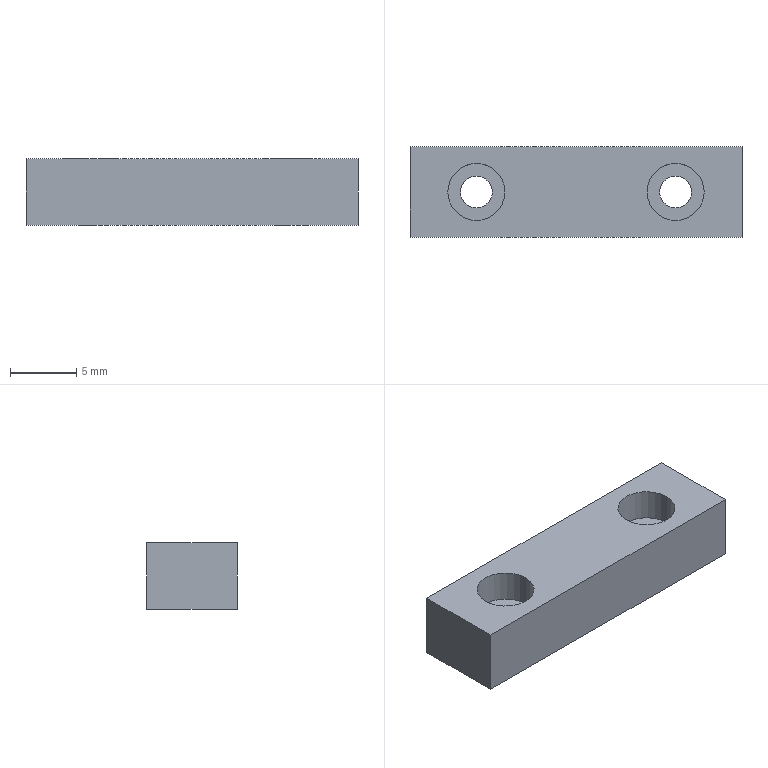Part | SolidWorks | features ICE 2, Extrusion 1 | 1 solid | 16 faces | box 25 x 6.8 x 5 mm | volume 756.77 mm3 | cylinder 8 | plane 8 | commonest cylinder face diameters 2.4 x4 4.3 x4
STEP:
#1=CARTESIAN_POINT('',(9.505,-0.3606,2.6));
#2=VERTEX_POINT('',#1);
#3=CARTESIAN_POINT('',(13.805,-0.3606,2.6));
#4=VERTEX_POINT('',#3);
#5=CARTESIAN_POINT('',(11.655,-0.3606,2.6));
#6=DIRECTION('',(0.,0.,1.));
#7=DIRECTION('',(1.,0.,0.));
#8=AXIS2_PLACEMENT_3D('',#5,#6,#7);
#9=CIRCLE('',#8,2.15);
#10=EDGE_CURVE('',#2,#4,#9,.T.);
#11=ORIENTED_EDGE('',*,*,#10,.F.);
#12=CARTESIAN_POINT('',(9.505,-0.3606,5.));
#13=VERTEX_POINT('',#12);
#14=CARTESIAN_POINT('',(9.505,-0.3606,2.6));
#15=DIRECTION('',(0.,0.,1.));
#16=VECTOR('',#15,1000.);
#17=LINE('',#14,#16);
#18=EDGE_CURVE('',#2,#13,#17,.T.);
#19=ORIENTED_EDGE('',*,*,#18,.T.);
#20=CARTESIAN_POINT('',(13.805,-0.3606,5.));
#21=VERTEX_POINT('',#20);
#22=CARTESIAN_POINT('',(11.655,-0.3606,5.));
#23=DIRECTION('',(0.,0.,1.));
#24=DIRECTION('',(1.,0.,0.));
#25=AXIS2_PLACEMENT_3D('',#22,#23,#24);
#26=CIRCLE('',#25,2.15);
#27=EDGE_CURVE('',#13,#21,#26,.T.);
#28=ORIENTED_EDGE('',*,*,#27,.T.);
#29=CARTESIAN_POINT('',(13.805,-0.3606,2.6));
#30=DIRECTION('',(0.,0.,1.));
#31=VECTOR('',#30,1000.);
#32=LINE('',#29,#31);
#33=EDGE_CURVE('',#4,#21,#32,.T.);
#34=ORIENTED_EDGE('',*,*,#33,.F.);
#35=EDGE_LOOP('',(#11,#19,#28,#34));
#36=FACE_OUTER_BOUND('',#35,.T.);
#37=CARTESIAN_POINT('',(11.655,-0.3606,2.6));
#38=DIRECTION('',(0.,0.,1.));
#39=DIRECTION('',(1.,0.,0.));
#40=AXIS2_PLACEMENT_3D('',#37,#38,#39);
#41=CYLINDRICAL_SURFACE('',#40,2.15);
#42=ADVANCED_FACE('',(#36),#41,.F.);
#43=CARTESIAN_POINT('',(-5.495,-0.3606,2.6));
#44=VERTEX_POINT('',#43);
#45=CARTESIAN_POINT('',(-1.195,-0.3606,2.6));
#46=VERTEX_POINT('',#45);
#47=CARTESIAN_POINT('',(-3.345,-0.3606,2.6));
#48=DIRECTION('',(0.,0.,1.));
#49=DIRECTION('',(1.,0.,0.));
#50=AXIS2_PLACEMENT_3D('',#47,#48,#49);
#51=CIRCLE('',#50,2.15);
#52=EDGE_CURVE('',#44,#46,#51,.T.);
#53=ORIENTED_EDGE('',*,*,#52,.F.);
#54=CARTESIAN_POINT('',(-5.495,-0.3606,5.));
#55=VERTEX_POINT('',#54);
#56=CARTESIAN_POINT('',(-5.495,-0.3606,2.6));
#57=DIRECTION('',(0.,0.,1.));
#58=VECTOR('',#57,1000.);
#59=LINE('',#56,#58);
#60=EDGE_CURVE('',#44,#55,#59,.T.);
#61=ORIENTED_EDGE('',*,*,#60,.T.);
#62=CARTESIAN_POINT('',(-1.195,-0.3606,5.));
#63=VERTEX_POINT('',#62);
#64=CARTESIAN_POINT('',(-3.345,-0.3606,5.));
#65=DIRECTION('',(0.,0.,1.));
#66=DIRECTION('',(1.,0.,0.));
#67=AXIS2_PLACEMENT_3D('',#64,#65,#66);
#68=CIRCLE('',#67,2.15);
#69=EDGE_CURVE('',#55,#63,#68,.T.);
#70=ORIENTED_EDGE('',*,*,#69,.T.);
#71=CARTESIAN_POINT('',(-1.195,-0.3606,2.6));
#72=DIRECTION('',(0.,0.,1.));
#73=VECTOR('',#72,1000.);
#74=LINE('',#71,#73);
#75=EDGE_CURVE('',#46,#63,#74,.T.);
#76=ORIENTED_EDGE('',*,*,#75,.F.);
#77=EDGE_LOOP('',(#53,#61,#70,#76));
#78=FACE_OUTER_BOUND('',#77,.T.);
#79=CARTESIAN_POINT('',(-3.345,-0.3606,2.6));
#80=DIRECTION('',(0.,0.,1.));
#81=DIRECTION('',(1.,0.,0.));
#82=AXIS2_PLACEMENT_3D('',#79,#80,#81);
#83=CYLINDRICAL_SURFACE('',#82,2.15);
#84=ADVANCED_FACE('',(#78),#83,.F.);
#85=CARTESIAN_POINT('',(-2.145,-0.3606,0.));
#86=VERTEX_POINT('',#85);
#87=CARTESIAN_POINT('',(-4.545,-0.3606,0.));
#88=VERTEX_POINT('',#87);
#89=CARTESIAN_POINT('',(-3.345,-0.3606,0.));
#90=DIRECTION('',(0.,0.,-1.));
#91=DIRECTION('',(1.,0.,0.));
#92=AXIS2_PLACEMENT_3D('',#89,#90,#91);
#93=CIRCLE('',#92,1.2);
#94=EDGE_CURVE('',#86,#88,#93,.T.);
#95=ORIENTED_EDGE('',*,*,#94,.T.);
#96=CARTESIAN_POINT('',(-4.545,-0.3606,2.6));
#97=VERTEX_POINT('',#96);
#98=CARTESIAN_POINT('',(-4.545,-0.3606,-0.001));
#99=DIRECTION('',(0.,0.,1.));
#100=VECTOR('',#99,1000.);
#101=LINE('',#98,#100);
#102=EDGE_CURVE('',#88,#97,#101,.T.);
#103=ORIENTED_EDGE('',*,*,#102,.T.);
#104=CARTESIAN_POINT('',(-2.145,-0.3606,2.6));
#105=VERTEX_POINT('',#104);
#106=CARTESIAN_POINT('',(-3.345,-0.3606,2.6));
#107=DIRECTION('',(0.,0.,-1.));
#108=DIRECTION('',(1.,0.,0.));
#109=AXIS2_PLACEMENT_3D('',#106,#107,#108);
#110=CIRCLE('',#109,1.2);
#111=EDGE_CURVE('',#105,#97,#110,.T.);
#112=ORIENTED_EDGE('',*,*,#111,.F.);
#113=CARTESIAN_POINT('',(-2.145,-0.3606,-0.001));
#114=DIRECTION('',(0.,0.,1.));
#115=VECTOR('',#114,1000.);
#116=LINE('',#113,#115);
#117=EDGE_CURVE('',#86,#105,#116,.T.);
#118=ORIENTED_EDGE('',*,*,#117,.F.);
#119=EDGE_LOOP('',(#95,#103,#112,#118));
#120=FACE_OUTER_BOUND('',#119,.T.);
#121=CARTESIAN_POINT('',(-3.345,-0.3606,-0.001));
#122=DIRECTION('',(0.,0.,1.));
#123=DIRECTION('',(1.,0.,0.));
#124=AXIS2_PLACEMENT_3D('',#121,#122,#123);
#125=CYLINDRICAL_SURFACE('',#124,1.2);
#126=ADVANCED_FACE('',(#120),#125,.F.);
#127=CARTESIAN_POINT('',(12.855,-0.3606,0.));
#128=VERTEX_POINT('',#127);
#129=CARTESIAN_POINT('',(10.455,-0.3606,0.));
#130=VERTEX_POINT('',#129);
#131=CARTESIAN_POINT('',(11.655,-0.3606,0.));
#132=DIRECTION('',(0.,0.,-1.));
#133=DIRECTION('',(1.,0.,0.));
#134=AXIS2_PLACEMENT_3D('',#131,#132,#133);
#135=CIRCLE('',#134,1.2);
#136=EDGE_CURVE('',#128,#130,#135,.T.);
#137=ORIENTED_EDGE('',*,*,#136,.T.);
#138=CARTESIAN_POINT('',(10.455,-0.3606,2.6));
#139=VERTEX_POINT('',#138);
#140=CARTESIAN_POINT('',(10.455,-0.3606,-0.001));
#141=DIRECTION('',(0.,0.,1.));
#142=VECTOR('',#141,1000.);
#143=LINE('',#140,#142);
#144=EDGE_CURVE('',#130,#139,#143,.T.);
#145=ORIENTED_EDGE('',*,*,#144,.T.);
#146=CARTESIAN_POINT('',(12.855,-0.3606,2.6));
#147=VERTEX_POINT('',#146);
#148=CARTESIAN_POINT('',(11.655,-0.3606,2.6));
#149=DIRECTION('',(0.,0.,-1.));
#150=DIRECTION('',(1.,0.,0.));
#151=AXIS2_PLACEMENT_3D('',#148,#149,#150);
#152=CIRCLE('',#151,1.2);
#153=EDGE_CURVE('',#147,#139,#152,.T.);
#154=ORIENTED_EDGE('',*,*,#153,.F.);
#155=CARTESIAN_POINT('',(12.855,-0.3606,-0.001));
#156=DIRECTION('',(0.,0.,1.));
#157=VECTOR('',#156,1000.);
#158=LINE('',#155,#157);
#159=EDGE_CURVE('',#128,#147,#158,.T.);
#160=ORIENTED_EDGE('',*,*,#159,.F.);
#161=EDGE_LOOP('',(#137,#145,#154,#160));
#162=FACE_OUTER_BOUND('',#161,.T.);
#163=CARTESIAN_POINT('',(11.655,-0.3606,-0.001));
#164=DIRECTION('',(0.,0.,1.));
#165=DIRECTION('',(1.,0.,0.));
#166=AXIS2_PLACEMENT_3D('',#163,#164,#165);
#167=CYLINDRICAL_SURFACE('',#166,1.2);
#168=ADVANCED_FACE('',(#162),#167,.F.);
#169=ORIENTED_EDGE('',*,*,#144,.F.);
#170=CARTESIAN_POINT('',(11.655,-0.3606,0.));
#171=DIRECTION('',(0.,0.,-1.));
#172=DIRECTION('',(1.,0.,0.));
#173=AXIS2_PLACEMENT_3D('',#170,#171,#172);
#174=CIRCLE('',#173,1.2);
#175=EDGE_CURVE('',#130,#128,#174,.T.);
#176=ORIENTED_EDGE('',*,*,#175,.T.);
#177=ORIENTED_EDGE('',*,*,#159,.T.);
#178=CARTESIAN_POINT('',(11.655,-0.3606,2.6));
#179=DIRECTION('',(0.,0.,-1.));
#180=DIRECTION('',(1.,0.,0.));
#181=AXIS2_PLACEMENT_3D('',#178,#179,#180);
#182=CIRCLE('',#181,1.2);
#183=EDGE_CURVE('',#139,#147,#182,.T.);
#184=ORIENTED_EDGE('',*,*,#183,.F.);
#185=EDGE_LOOP('',(#169,#176,#177,#184));
#186=FACE_OUTER_BOUND('',#185,.T.);
#187=CARTESIAN_POINT('',(11.655,-0.3606,-0.001));
#188=DIRECTION('',(0.,0.,1.));
#189=DIRECTION('',(1.,0.,0.));
#190=AXIS2_PLACEMENT_3D('',#187,#188,#189);
#191=CYLINDRICAL_SURFACE('',#190,1.2);
#192=ADVANCED_FACE('',(#186),#191,.F.);
#193=ORIENTED_EDGE('',*,*,#102,.F.);
#194=CARTESIAN_POINT('',(-3.345,-0.3606,0.));
#195=DIRECTION('',(0.,0.,-1.));
#196=DIRECTION('',(1.,0.,0.));
#197=AXIS2_PLACEMENT_3D('',#194,#195,#196);
#198=CIRCLE('',#197,1.2);
#199=EDGE_CURVE('',#88,#86,#198,.T.);
#200=ORIENTED_EDGE('',*,*,#199,.T.);
#201=ORIENTED_EDGE('',*,*,#117,.T.);
#202=CARTESIAN_POINT('',(-3.345,-0.3606,2.6));
#203=DIRECTION('',(0.,0.,-1.));
#204=DIRECTION('',(1.,0.,0.));
#205=AXIS2_PLACEMENT_3D('',#202,#203,#204);
#206=CIRCLE('',#205,1.2);
#207=EDGE_CURVE('',#97,#105,#206,.T.);
#208=ORIENTED_EDGE('',*,*,#207,.F.);
#209=EDGE_LOOP('',(#193,#200,#201,#208));
#210=FACE_OUTER_BOUND('',#209,.T.);
#211=CARTESIAN_POINT('',(-3.345,-0.3606,-0.001));
#212=DIRECTION('',(0.,0.,1.));
#213=DIRECTION('',(1.,0.,0.));
#214=AXIS2_PLACEMENT_3D('',#211,#212,#213);
#215=CYLINDRICAL_SURFACE('',#214,1.2);
#216=ADVANCED_FACE('',(#210),#215,.F.);
#217=CARTESIAN_POINT('',(-8.345,3.039,0.));
#218=VERTEX_POINT('',#217);
#219=CARTESIAN_POINT('',(-8.345,-3.761,0.));
#220=VERTEX_POINT('',#219);
#221=CARTESIAN_POINT('',(-8.345,3.039,0.));
#222=DIRECTION('',(0.,-1.,0.));
#223=VECTOR('',#222,1000.);
#224=LINE('',#221,#223);
#225=EDGE_CURVE('',#218,#220,#224,.T.);
#226=ORIENTED_EDGE('',*,*,#225,.T.);
#227=CARTESIAN_POINT('',(-8.345,-3.761,5.));
#228=VERTEX_POINT('',#227);
#229=CARTESIAN_POINT('',(-8.345,-3.761,5.));
#230=DIRECTION('',(0.,0.,-1.));
#231=VECTOR('',#230,1000.);
#232=LINE('',#229,#231);
#233=EDGE_CURVE('',#228,#220,#232,.T.);
#234=ORIENTED_EDGE('',*,*,#233,.F.);
#235=CARTESIAN_POINT('',(-8.345,3.039,5.));
#236=VERTEX_POINT('',#235);
#237=CARTESIAN_POINT('',(-8.345,3.039,5.));
#238=DIRECTION('',(0.,-1.,0.));
#239=VECTOR('',#238,1000.);
#240=LINE('',#237,#239);
#241=EDGE_CURVE('',#236,#228,#240,.T.);
#242=ORIENTED_EDGE('',*,*,#241,.F.);
#243=CARTESIAN_POINT('',(-8.345,3.039,5.));
#244=DIRECTION('',(0.,0.,-1.));
#245=VECTOR('',#244,1000.);
#246=LINE('',#243,#245);
#247=EDGE_CURVE('',#236,#218,#246,.T.);
#248=ORIENTED_EDGE('',*,*,#247,.T.);
#249=EDGE_LOOP('',(#226,#234,#242,#248));
#250=FACE_OUTER_BOUND('',#249,.T.);
#251=CARTESIAN_POINT('',(-8.345,3.039,5.));
#252=DIRECTION('',(1.,0.,0.));
#253=DIRECTION('',(0.,0.,-1.));
#254=AXIS2_PLACEMENT_3D('',#251,#252,#253);
#255=PLANE('',#254);
#256=ADVANCED_FACE('',(#250),#255,.F.);
#257=CARTESIAN_POINT('',(16.655,-3.761,0.));
#258=VERTEX_POINT('',#257);
#259=CARTESIAN_POINT('',(-8.345,-3.761,0.));
#260=DIRECTION('',(1.,0.,0.));
#261=VECTOR('',#260,1000.);
#262=LINE('',#259,#261);
#263=EDGE_CURVE('',#220,#258,#262,.T.);
#264=ORIENTED_EDGE('',*,*,#263,.T.);
#265=CARTESIAN_POINT('',(16.655,-3.761,5.));
#266=VERTEX_POINT('',#265);
#267=CARTESIAN_POINT('',(16.655,-3.761,5.));
#268=DIRECTION('',(0.,0.,-1.));
#269=VECTOR('',#268,1000.);
#270=LINE('',#267,#269);
#271=EDGE_CURVE('',#266,#258,#270,.T.);
#272=ORIENTED_EDGE('',*,*,#271,.F.);
#273=CARTESIAN_POINT('',(-8.345,-3.761,5.));
#274=DIRECTION('',(1.,0.,0.));
#275=VECTOR('',#274,1000.);
#276=LINE('',#273,#275);
#277=EDGE_CURVE('',#228,#266,#276,.T.);
#278=ORIENTED_EDGE('',*,*,#277,.F.);
#279=ORIENTED_EDGE('',*,*,#233,.T.);
#280=EDGE_LOOP('',(#264,#272,#278,#279));
#281=FACE_OUTER_BOUND('',#280,.T.);
#282=CARTESIAN_POINT('',(-8.345,-3.761,5.));
#283=DIRECTION('',(0.,1.,0.));
#284=DIRECTION('',(-1.,0.,0.));
#285=AXIS2_PLACEMENT_3D('',#282,#283,#284);
#286=PLANE('',#285);
#287=ADVANCED_FACE('',(#281),#286,.F.);
#288=CARTESIAN_POINT('',(16.655,3.039,0.));
#289=VERTEX_POINT('',#288);
#290=CARTESIAN_POINT('',(16.655,3.039,0.));
#291=DIRECTION('',(0.,1.,0.));
#292=VECTOR('',#291,1000.);
#293=LINE('',#290,#292);
#294=EDGE_CURVE('',#258,#289,#293,.T.);
#295=ORIENTED_EDGE('',*,*,#294,.T.);
#296=CARTESIAN_POINT('',(16.655,3.039,5.));
#297=VERTEX_POINT('',#296);
#298=CARTESIAN_POINT('',(16.655,3.039,5.));
#299=DIRECTION('',(0.,0.,-1.));
#300=VECTOR('',#299,1000.);
#301=LINE('',#298,#300);
#302=EDGE_CURVE('',#297,#289,#301,.T.);
#303=ORIENTED_EDGE('',*,*,#302,.F.);
#304=CARTESIAN_POINT('',(16.655,3.039,5.));
#305=DIRECTION('',(0.,1.,0.));
#306=VECTOR('',#305,1000.);
#307=LINE('',#304,#306);
#308=EDGE_CURVE('',#266,#297,#307,.T.);
#309=ORIENTED_EDGE('',*,*,#308,.F.);
#310=ORIENTED_EDGE('',*,*,#271,.T.);
#311=EDGE_LOOP('',(#295,#303,#309,#310));
#312=FACE_OUTER_BOUND('',#311,.T.);
#313=CARTESIAN_POINT('',(16.655,3.039,5.));
#314=DIRECTION('',(-1.,0.,0.));
#315=DIRECTION('',(0.,0.,1.));
#316=AXIS2_PLACEMENT_3D('',#313,#314,#315);
#317=PLANE('',#316);
#318=ADVANCED_FACE('',(#312),#317,.F.);
#319=CARTESIAN_POINT('',(-8.345,3.039,0.));
#320=DIRECTION('',(-1.,0.,0.));
#321=VECTOR('',#320,1000.);
#322=LINE('',#319,#321);
#323=EDGE_CURVE('',#289,#218,#322,.T.);
#324=ORIENTED_EDGE('',*,*,#323,.T.);
#325=ORIENTED_EDGE('',*,*,#247,.F.);
#326=CARTESIAN_POINT('',(-8.345,3.039,5.));
#327=DIRECTION('',(-1.,0.,0.));
#328=VECTOR('',#327,1000.);
#329=LINE('',#326,#328);
#330=EDGE_CURVE('',#297,#236,#329,.T.);
#331=ORIENTED_EDGE('',*,*,#330,.F.);
#332=ORIENTED_EDGE('',*,*,#302,.T.);
#333=EDGE_LOOP('',(#324,#325,#331,#332));
#334=FACE_OUTER_BOUND('',#333,.T.);
#335=CARTESIAN_POINT('',(-8.345,3.039,5.));
#336=DIRECTION('',(0.,-1.,0.));
#337=DIRECTION('',(0.,0.,-1.));
#338=AXIS2_PLACEMENT_3D('',#335,#336,#337);
#339=PLANE('',#338);
#340=ADVANCED_FACE('',(#334),#339,.F.);
#341=CARTESIAN_POINT('',(-3.345,-0.3606,5.));
#342=DIRECTION('',(0.,0.,1.));
#343=DIRECTION('',(1.,0.,0.));
#344=AXIS2_PLACEMENT_3D('',#341,#342,#343);
#345=CIRCLE('',#344,2.15);
#346=EDGE_CURVE('',#63,#55,#345,.T.);
#347=ORIENTED_EDGE('',*,*,#346,.F.);
#348=ORIENTED_EDGE('',*,*,#69,.F.);
#349=EDGE_LOOP('',(#347,#348));
#350=FACE_BOUND('',#349,.T.);
#351=CARTESIAN_POINT('',(11.655,-0.3606,5.));
#352=DIRECTION('',(0.,0.,1.));
#353=DIRECTION('',(1.,0.,0.));
#354=AXIS2_PLACEMENT_3D('',#351,#352,#353);
#355=CIRCLE('',#354,2.15);
#356=EDGE_CURVE('',#21,#13,#355,.T.);
#357=ORIENTED_EDGE('',*,*,#356,.F.);
#358=ORIENTED_EDGE('',*,*,#27,.F.);
#359=EDGE_LOOP('',(#357,#358));
#360=FACE_BOUND('',#359,.T.);
#361=ORIENTED_EDGE('',*,*,#241,.T.);
#362=ORIENTED_EDGE('',*,*,#277,.T.);
#363=ORIENTED_EDGE('',*,*,#308,.T.);
#364=ORIENTED_EDGE('',*,*,#330,.T.);
#365=EDGE_LOOP('',(#361,#362,#363,#364));
#366=FACE_OUTER_BOUND('',#365,.T.);
#367=CARTESIAN_POINT('',(0.,0.,5.));
#368=DIRECTION('',(0.,0.,1.));
#369=DIRECTION('',(1.,0.,0.));
#370=AXIS2_PLACEMENT_3D('',#367,#368,#369);
#371=PLANE('',#370);
#372=ADVANCED_FACE('',(#350,#360,#366),#371,.T.);
#373=ORIENTED_EDGE('',*,*,#94,.F.);
#374=ORIENTED_EDGE('',*,*,#199,.F.);
#375=EDGE_LOOP('',(#373,#374));
#376=FACE_BOUND('',#375,.T.);
#377=ORIENTED_EDGE('',*,*,#136,.F.);
#378=ORIENTED_EDGE('',*,*,#175,.F.);
#379=EDGE_LOOP('',(#377,#378));
#380=FACE_BOUND('',#379,.T.);
#381=ORIENTED_EDGE('',*,*,#225,.F.);
#382=ORIENTED_EDGE('',*,*,#323,.F.);
#383=ORIENTED_EDGE('',*,*,#294,.F.);
#384=ORIENTED_EDGE('',*,*,#263,.F.);
#385=EDGE_LOOP('',(#381,#382,#383,#384));
#386=FACE_OUTER_BOUND('',#385,.T.);
#387=CARTESIAN_POINT('',(0.,0.,0.));
#388=DIRECTION('',(0.,0.,1.));
#389=DIRECTION('',(1.,0.,0.));
#390=AXIS2_PLACEMENT_3D('',#387,#388,#389);
#391=PLANE('',#390);
#392=ADVANCED_FACE('',(#376,#380,#386),#391,.F.);
#393=CARTESIAN_POINT('',(-3.345,-0.3606,2.6));
#394=DIRECTION('',(0.,0.,1.));
#395=DIRECTION('',(1.,0.,0.));
#396=AXIS2_PLACEMENT_3D('',#393,#394,#395);
#397=CIRCLE('',#396,2.15);
#398=EDGE_CURVE('',#46,#44,#397,.T.);
#399=ORIENTED_EDGE('',*,*,#398,.T.);
#400=ORIENTED_EDGE('',*,*,#52,.T.);
#401=EDGE_LOOP('',(#399,#400));
#402=FACE_OUTER_BOUND('',#401,.T.);
#403=ORIENTED_EDGE('',*,*,#111,.T.);
#404=ORIENTED_EDGE('',*,*,#207,.T.);
#405=EDGE_LOOP('',(#403,#404));
#406=FACE_BOUND('',#405,.T.);
#407=CARTESIAN_POINT('',(-3.345,-0.3606,2.6));
#408=DIRECTION('',(0.,0.,1.));
#409=DIRECTION('',(1.,0.,0.));
#410=AXIS2_PLACEMENT_3D('',#407,#408,#409);
#411=PLANE('',#410);
#412=ADVANCED_FACE('',(#402,#406),#411,.T.);
#413=ORIENTED_EDGE('',*,*,#60,.F.);
#414=ORIENTED_EDGE('',*,*,#398,.F.);
#415=ORIENTED_EDGE('',*,*,#75,.T.);
#416=ORIENTED_EDGE('',*,*,#346,.T.);
#417=EDGE_LOOP('',(#413,#414,#415,#416));
#418=FACE_OUTER_BOUND('',#417,.T.);
#419=CARTESIAN_POINT('',(-3.345,-0.3606,2.6));
#420=DIRECTION('',(0.,0.,1.));
#421=DIRECTION('',(1.,0.,0.));
#422=AXIS2_PLACEMENT_3D('',#419,#420,#421);
#423=CYLINDRICAL_SURFACE('',#422,2.15);
#424=ADVANCED_FACE('',(#418),#423,.F.);
#425=CARTESIAN_POINT('',(11.655,-0.3606,2.6));
#426=DIRECTION('',(0.,0.,1.));
#427=DIRECTION('',(1.,0.,0.));
#428=AXIS2_PLACEMENT_3D('',#425,#426,#427);
#429=CIRCLE('',#428,2.15);
#430=EDGE_CURVE('',#4,#2,#429,.T.);
#431=ORIENTED_EDGE('',*,*,#430,.T.);
#432=ORIENTED_EDGE('',*,*,#10,.T.);
#433=EDGE_LOOP('',(#431,#432));
#434=FACE_OUTER_BOUND('',#433,.T.);
#435=ORIENTED_EDGE('',*,*,#153,.T.);
#436=ORIENTED_EDGE('',*,*,#183,.T.);
#437=EDGE_LOOP('',(#435,#436));
#438=FACE_BOUND('',#437,.T.);
#439=CARTESIAN_POINT('',(11.655,-0.3606,2.6));
#440=DIRECTION('',(0.,0.,1.));
#441=DIRECTION('',(1.,0.,0.));
#442=AXIS2_PLACEMENT_3D('',#439,#440,#441);
#443=PLANE('',#442);
#444=ADVANCED_FACE('',(#434,#438),#443,.T.);
#445=ORIENTED_EDGE('',*,*,#18,.F.);
#446=ORIENTED_EDGE('',*,*,#430,.F.);
#447=ORIENTED_EDGE('',*,*,#33,.T.);
#448=ORIENTED_EDGE('',*,*,#356,.T.);
#449=EDGE_LOOP('',(#445,#446,#447,#448));
#450=FACE_OUTER_BOUND('',#449,.T.);
#451=CARTESIAN_POINT('',(11.655,-0.3606,2.6));
#452=DIRECTION('',(0.,0.,1.));
#453=DIRECTION('',(1.,0.,0.));
#454=AXIS2_PLACEMENT_3D('',#451,#452,#453);
#455=CYLINDRICAL_SURFACE('',#454,2.15);
#456=ADVANCED_FACE('',(#450),#455,.F.);
#457=CLOSED_SHELL('',(#42,#84,#126,#168,#192,#216,#256,#287,#318,#340,#372,#392,#412,#424,#444,#456));
#458=MANIFOLD_SOLID_BREP('',#457);
#459=CARTESIAN_POINT('',(0.,0.,0.));
#460=DIRECTION('',(0.,0.,1.));
#461=DIRECTION('',(1.,0.,0.));
#462=AXIS2_PLACEMENT_3D('',#459,#460,#461);
#463=(LENGTH_UNIT()NAMED_UNIT(*)SI_UNIT(.MILLI.,.METRE.));
#464=UNCERTAINTY_MEASURE_WITH_UNIT(LENGTH_MEASURE(0.00001),#463,'','');
#465=(NAMED_UNIT(*)PLANE_ANGLE_UNIT()SI_UNIT($,.RADIAN.));
#466=(NAMED_UNIT(*)SI_UNIT($,.STERADIAN.)SOLID_ANGLE_UNIT());
#467=(GEOMETRIC_REPRESENTATION_CONTEXT(3)GLOBAL_UNCERTAINTY_ASSIGNED_CONTEXT((#464))GLOBAL_UNIT_ASSIGNED_CONTEXT((#463,#465,#466))REPRESENTATION_CONTEXT('',''));
#468=ADVANCED_BREP_SHAPE_REPRESENTATION('',(#458,#462),#467);